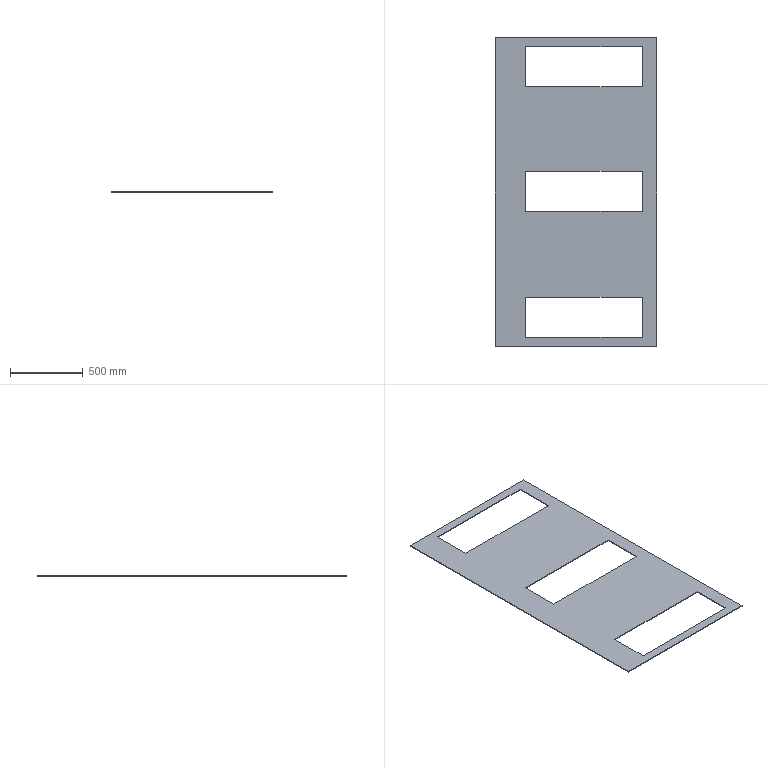Part | SolidWorks | features Extrusion 1 | 1 solid | 18 faces | box 1111 x 2124 x 5 mm | volume 8464783 mm3 | plane 18
STEP:
#1=CARTESIAN_POINT('',(207.052,1206.44,5.));
#2=VERTEX_POINT('',#1);
#3=CARTESIAN_POINT('',(207.052,930.678,5.));
#4=VERTEX_POINT('',#3);
#5=CARTESIAN_POINT('',(207.052,930.678,5.));
#6=DIRECTION('',(0.,-1.,0.));
#7=VECTOR('',#6,1000.);
#8=LINE('',#5,#7);
#9=EDGE_CURVE('',#2,#4,#8,.T.);
#10=ORIENTED_EDGE('',*,*,#9,.F.);
#11=CARTESIAN_POINT('',(1012.074,1206.44,5.));
#12=VERTEX_POINT('',#11);
#13=CARTESIAN_POINT('',(207.052,1206.44,5.));
#14=DIRECTION('',(-1.,0.,0.));
#15=VECTOR('',#14,1000.);
#16=LINE('',#13,#15);
#17=EDGE_CURVE('',#12,#2,#16,.T.);
#18=ORIENTED_EDGE('',*,*,#17,.F.);
#19=CARTESIAN_POINT('',(1012.074,930.678,5.));
#20=VERTEX_POINT('',#19);
#21=CARTESIAN_POINT('',(1012.074,1206.44,5.));
#22=DIRECTION('',(0.,1.,0.));
#23=VECTOR('',#22,1000.);
#24=LINE('',#21,#23);
#25=EDGE_CURVE('',#20,#12,#24,.T.);
#26=ORIENTED_EDGE('',*,*,#25,.F.);
#27=CARTESIAN_POINT('',(1012.074,930.678,5.));
#28=DIRECTION('',(1.,0.,0.));
#29=VECTOR('',#28,1000.);
#30=LINE('',#27,#29);
#31=EDGE_CURVE('',#4,#20,#30,.T.);
#32=ORIENTED_EDGE('',*,*,#31,.F.);
#33=EDGE_LOOP('',(#10,#18,#26,#32));
#34=FACE_BOUND('',#33,.T.);
#35=CARTESIAN_POINT('',(0.,2124.,5.));
#36=VERTEX_POINT('',#35);
#37=CARTESIAN_POINT('',(0.,0.,5.));
#38=VERTEX_POINT('',#37);
#39=CARTESIAN_POINT('',(0.,0.,5.));
#40=DIRECTION('',(0.,-1.,0.));
#41=VECTOR('',#40,1000.);
#42=LINE('',#39,#41);
#43=EDGE_CURVE('',#36,#38,#42,.T.);
#44=ORIENTED_EDGE('',*,*,#43,.T.);
#45=CARTESIAN_POINT('',(1110.612,0.,5.));
#46=VERTEX_POINT('',#45);
#47=CARTESIAN_POINT('',(1110.612,0.,5.));
#48=DIRECTION('',(1.,0.,0.));
#49=VECTOR('',#48,1000.);
#50=LINE('',#47,#49);
#51=EDGE_CURVE('',#38,#46,#50,.T.);
#52=ORIENTED_EDGE('',*,*,#51,.T.);
#53=CARTESIAN_POINT('',(1110.612,2124.,5.));
#54=VERTEX_POINT('',#53);
#55=CARTESIAN_POINT('',(1110.612,2124.,5.));
#56=DIRECTION('',(0.,1.,0.));
#57=VECTOR('',#56,1000.);
#58=LINE('',#55,#57);
#59=EDGE_CURVE('',#46,#54,#58,.T.);
#60=ORIENTED_EDGE('',*,*,#59,.T.);
#61=CARTESIAN_POINT('',(0.,2124.,5.));
#62=DIRECTION('',(-1.,0.,0.));
#63=VECTOR('',#62,1000.);
#64=LINE('',#61,#63);
#65=EDGE_CURVE('',#54,#36,#64,.T.);
#66=ORIENTED_EDGE('',*,*,#65,.T.);
#67=EDGE_LOOP('',(#44,#52,#60,#66));
#68=FACE_OUTER_BOUND('',#67,.T.);
#69=CARTESIAN_POINT('',(207.052,2063.657,5.));
#70=VERTEX_POINT('',#69);
#71=CARTESIAN_POINT('',(207.052,1787.895,5.));
#72=VERTEX_POINT('',#71);
#73=CARTESIAN_POINT('',(207.052,1787.895,5.));
#74=DIRECTION('',(0.,-1.,0.));
#75=VECTOR('',#74,1000.);
#76=LINE('',#73,#75);
#77=EDGE_CURVE('',#70,#72,#76,.T.);
#78=ORIENTED_EDGE('',*,*,#77,.F.);
#79=CARTESIAN_POINT('',(1012.074,2063.657,5.));
#80=VERTEX_POINT('',#79);
#81=CARTESIAN_POINT('',(207.052,2063.657,5.));
#82=DIRECTION('',(-1.,0.,0.));
#83=VECTOR('',#82,1000.);
#84=LINE('',#81,#83);
#85=EDGE_CURVE('',#80,#70,#84,.T.);
#86=ORIENTED_EDGE('',*,*,#85,.F.);
#87=CARTESIAN_POINT('',(1012.074,1787.895,5.));
#88=VERTEX_POINT('',#87);
#89=CARTESIAN_POINT('',(1012.074,2063.657,5.));
#90=DIRECTION('',(0.,1.,0.));
#91=VECTOR('',#90,1000.);
#92=LINE('',#89,#91);
#93=EDGE_CURVE('',#88,#80,#92,.T.);
#94=ORIENTED_EDGE('',*,*,#93,.F.);
#95=CARTESIAN_POINT('',(1012.074,1787.895,5.));
#96=DIRECTION('',(1.,0.,0.));
#97=VECTOR('',#96,1000.);
#98=LINE('',#95,#97);
#99=EDGE_CURVE('',#72,#88,#98,.T.);
#100=ORIENTED_EDGE('',*,*,#99,.F.);
#101=EDGE_LOOP('',(#78,#86,#94,#100));
#102=FACE_BOUND('',#101,.T.);
#103=CARTESIAN_POINT('',(207.052,336.013,5.));
#104=VERTEX_POINT('',#103);
#105=CARTESIAN_POINT('',(207.052,60.251,5.));
#106=VERTEX_POINT('',#105);
#107=CARTESIAN_POINT('',(207.052,60.251,5.));
#108=DIRECTION('',(0.,-1.,0.));
#109=VECTOR('',#108,1000.);
#110=LINE('',#107,#109);
#111=EDGE_CURVE('',#104,#106,#110,.T.);
#112=ORIENTED_EDGE('',*,*,#111,.F.);
#113=CARTESIAN_POINT('',(1012.074,336.013,5.));
#114=VERTEX_POINT('',#113);
#115=CARTESIAN_POINT('',(207.052,336.013,5.));
#116=DIRECTION('',(-1.,0.,0.));
#117=VECTOR('',#116,1000.);
#118=LINE('',#115,#117);
#119=EDGE_CURVE('',#114,#104,#118,.T.);
#120=ORIENTED_EDGE('',*,*,#119,.F.);
#121=CARTESIAN_POINT('',(1012.074,60.251,5.));
#122=VERTEX_POINT('',#121);
#123=CARTESIAN_POINT('',(1012.074,336.013,5.));
#124=DIRECTION('',(0.,1.,0.));
#125=VECTOR('',#124,1000.);
#126=LINE('',#123,#125);
#127=EDGE_CURVE('',#122,#114,#126,.T.);
#128=ORIENTED_EDGE('',*,*,#127,.F.);
#129=CARTESIAN_POINT('',(1012.074,60.251,5.));
#130=DIRECTION('',(1.,0.,0.));
#131=VECTOR('',#130,1000.);
#132=LINE('',#129,#131);
#133=EDGE_CURVE('',#106,#122,#132,.T.);
#134=ORIENTED_EDGE('',*,*,#133,.F.);
#135=EDGE_LOOP('',(#112,#120,#128,#134));
#136=FACE_BOUND('',#135,.T.);
#137=CARTESIAN_POINT('',(0.,0.,5.));
#138=DIRECTION('',(0.,0.,-1.));
#139=DIRECTION('',(-1.,0.,0.));
#140=AXIS2_PLACEMENT_3D('',#137,#138,#139);
#141=PLANE('',#140);
#142=ADVANCED_FACE('',(#34,#68,#102,#136),#141,.F.);
#143=CARTESIAN_POINT('',(0.,2124.,0.));
#144=VERTEX_POINT('',#143);
#145=CARTESIAN_POINT('',(0.,0.,0.));
#146=VERTEX_POINT('',#145);
#147=CARTESIAN_POINT('',(0.,0.,0.));
#148=DIRECTION('',(0.,-1.,0.));
#149=VECTOR('',#148,1000.);
#150=LINE('',#147,#149);
#151=EDGE_CURVE('',#144,#146,#150,.T.);
#152=ORIENTED_EDGE('',*,*,#151,.F.);
#153=CARTESIAN_POINT('',(1110.612,2124.,0.));
#154=VERTEX_POINT('',#153);
#155=CARTESIAN_POINT('',(0.,2124.,0.));
#156=DIRECTION('',(-1.,0.,0.));
#157=VECTOR('',#156,1000.);
#158=LINE('',#155,#157);
#159=EDGE_CURVE('',#154,#144,#158,.T.);
#160=ORIENTED_EDGE('',*,*,#159,.F.);
#161=CARTESIAN_POINT('',(1110.612,0.,0.));
#162=VERTEX_POINT('',#161);
#163=CARTESIAN_POINT('',(1110.612,2124.,0.));
#164=DIRECTION('',(0.,1.,0.));
#165=VECTOR('',#164,1000.);
#166=LINE('',#163,#165);
#167=EDGE_CURVE('',#162,#154,#166,.T.);
#168=ORIENTED_EDGE('',*,*,#167,.F.);
#169=CARTESIAN_POINT('',(1110.612,0.,0.));
#170=DIRECTION('',(1.,0.,0.));
#171=VECTOR('',#170,1000.);
#172=LINE('',#169,#171);
#173=EDGE_CURVE('',#146,#162,#172,.T.);
#174=ORIENTED_EDGE('',*,*,#173,.F.);
#175=EDGE_LOOP('',(#152,#160,#168,#174));
#176=FACE_OUTER_BOUND('',#175,.T.);
#177=CARTESIAN_POINT('',(1012.074,2063.657,0.));
#178=VERTEX_POINT('',#177);
#179=CARTESIAN_POINT('',(207.052,2063.657,0.));
#180=VERTEX_POINT('',#179);
#181=CARTESIAN_POINT('',(207.052,2063.657,0.));
#182=DIRECTION('',(-1.,0.,0.));
#183=VECTOR('',#182,1000.);
#184=LINE('',#181,#183);
#185=EDGE_CURVE('',#178,#180,#184,.T.);
#186=ORIENTED_EDGE('',*,*,#185,.T.);
#187=CARTESIAN_POINT('',(207.052,1787.895,0.));
#188=VERTEX_POINT('',#187);
#189=CARTESIAN_POINT('',(207.052,1787.895,0.));
#190=DIRECTION('',(0.,-1.,0.));
#191=VECTOR('',#190,1000.);
#192=LINE('',#189,#191);
#193=EDGE_CURVE('',#180,#188,#192,.T.);
#194=ORIENTED_EDGE('',*,*,#193,.T.);
#195=CARTESIAN_POINT('',(1012.074,1787.895,0.));
#196=VERTEX_POINT('',#195);
#197=CARTESIAN_POINT('',(1012.074,1787.895,0.));
#198=DIRECTION('',(1.,0.,0.));
#199=VECTOR('',#198,1000.);
#200=LINE('',#197,#199);
#201=EDGE_CURVE('',#188,#196,#200,.T.);
#202=ORIENTED_EDGE('',*,*,#201,.T.);
#203=CARTESIAN_POINT('',(1012.074,2063.657,0.));
#204=DIRECTION('',(0.,1.,0.));
#205=VECTOR('',#204,1000.);
#206=LINE('',#203,#205);
#207=EDGE_CURVE('',#196,#178,#206,.T.);
#208=ORIENTED_EDGE('',*,*,#207,.T.);
#209=EDGE_LOOP('',(#186,#194,#202,#208));
#210=FACE_BOUND('',#209,.T.);
#211=CARTESIAN_POINT('',(1012.074,1206.44,0.));
#212=VERTEX_POINT('',#211);
#213=CARTESIAN_POINT('',(207.052,1206.44,0.));
#214=VERTEX_POINT('',#213);
#215=CARTESIAN_POINT('',(207.052,1206.44,0.));
#216=DIRECTION('',(-1.,0.,0.));
#217=VECTOR('',#216,1000.);
#218=LINE('',#215,#217);
#219=EDGE_CURVE('',#212,#214,#218,.T.);
#220=ORIENTED_EDGE('',*,*,#219,.T.);
#221=CARTESIAN_POINT('',(207.052,930.678,0.));
#222=VERTEX_POINT('',#221);
#223=CARTESIAN_POINT('',(207.052,930.678,0.));
#224=DIRECTION('',(0.,-1.,0.));
#225=VECTOR('',#224,1000.);
#226=LINE('',#223,#225);
#227=EDGE_CURVE('',#214,#222,#226,.T.);
#228=ORIENTED_EDGE('',*,*,#227,.T.);
#229=CARTESIAN_POINT('',(1012.074,930.678,0.));
#230=VERTEX_POINT('',#229);
#231=CARTESIAN_POINT('',(1012.074,930.678,0.));
#232=DIRECTION('',(1.,0.,0.));
#233=VECTOR('',#232,1000.);
#234=LINE('',#231,#233);
#235=EDGE_CURVE('',#222,#230,#234,.T.);
#236=ORIENTED_EDGE('',*,*,#235,.T.);
#237=CARTESIAN_POINT('',(1012.074,1206.44,0.));
#238=DIRECTION('',(0.,1.,0.));
#239=VECTOR('',#238,1000.);
#240=LINE('',#237,#239);
#241=EDGE_CURVE('',#230,#212,#240,.T.);
#242=ORIENTED_EDGE('',*,*,#241,.T.);
#243=EDGE_LOOP('',(#220,#228,#236,#242));
#244=FACE_BOUND('',#243,.T.);
#245=CARTESIAN_POINT('',(1012.074,336.013,0.));
#246=VERTEX_POINT('',#245);
#247=CARTESIAN_POINT('',(207.052,336.013,0.));
#248=VERTEX_POINT('',#247);
#249=CARTESIAN_POINT('',(207.052,336.013,0.));
#250=DIRECTION('',(-1.,0.,0.));
#251=VECTOR('',#250,1000.);
#252=LINE('',#249,#251);
#253=EDGE_CURVE('',#246,#248,#252,.T.);
#254=ORIENTED_EDGE('',*,*,#253,.T.);
#255=CARTESIAN_POINT('',(207.052,60.251,0.));
#256=VERTEX_POINT('',#255);
#257=CARTESIAN_POINT('',(207.052,60.251,0.));
#258=DIRECTION('',(0.,-1.,0.));
#259=VECTOR('',#258,1000.);
#260=LINE('',#257,#259);
#261=EDGE_CURVE('',#248,#256,#260,.T.);
#262=ORIENTED_EDGE('',*,*,#261,.T.);
#263=CARTESIAN_POINT('',(1012.074,60.251,0.));
#264=VERTEX_POINT('',#263);
#265=CARTESIAN_POINT('',(1012.074,60.251,0.));
#266=DIRECTION('',(1.,0.,0.));
#267=VECTOR('',#266,1000.);
#268=LINE('',#265,#267);
#269=EDGE_CURVE('',#256,#264,#268,.T.);
#270=ORIENTED_EDGE('',*,*,#269,.T.);
#271=CARTESIAN_POINT('',(1012.074,336.013,0.));
#272=DIRECTION('',(0.,1.,0.));
#273=VECTOR('',#272,1000.);
#274=LINE('',#271,#273);
#275=EDGE_CURVE('',#264,#246,#274,.T.);
#276=ORIENTED_EDGE('',*,*,#275,.T.);
#277=EDGE_LOOP('',(#254,#262,#270,#276));
#278=FACE_BOUND('',#277,.T.);
#279=CARTESIAN_POINT('',(0.,0.,0.));
#280=DIRECTION('',(0.,0.,-1.));
#281=DIRECTION('',(-1.,0.,0.));
#282=AXIS2_PLACEMENT_3D('',#279,#280,#281);
#283=PLANE('',#282);
#284=ADVANCED_FACE('',(#176,#210,#244,#278),#283,.T.);
#285=ORIENTED_EDGE('',*,*,#151,.T.);
#286=CARTESIAN_POINT('',(0.,0.,5.));
#287=DIRECTION('',(0.,0.,-1.));
#288=VECTOR('',#287,1000.);
#289=LINE('',#286,#288);
#290=EDGE_CURVE('',#38,#146,#289,.T.);
#291=ORIENTED_EDGE('',*,*,#290,.F.);
#292=ORIENTED_EDGE('',*,*,#43,.F.);
#293=CARTESIAN_POINT('',(0.,2124.,5.));
#294=DIRECTION('',(0.,0.,-1.));
#295=VECTOR('',#294,1000.);
#296=LINE('',#293,#295);
#297=EDGE_CURVE('',#36,#144,#296,.T.);
#298=ORIENTED_EDGE('',*,*,#297,.T.);
#299=EDGE_LOOP('',(#285,#291,#292,#298));
#300=FACE_OUTER_BOUND('',#299,.T.);
#301=CARTESIAN_POINT('',(0.,0.,5.));
#302=DIRECTION('',(1.,0.,0.));
#303=DIRECTION('',(0.,0.,-1.));
#304=AXIS2_PLACEMENT_3D('',#301,#302,#303);
#305=PLANE('',#304);
#306=ADVANCED_FACE('',(#300),#305,.F.);
#307=ORIENTED_EDGE('',*,*,#173,.T.);
#308=CARTESIAN_POINT('',(1110.612,0.,5.));
#309=DIRECTION('',(0.,0.,-1.));
#310=VECTOR('',#309,1000.);
#311=LINE('',#308,#310);
#312=EDGE_CURVE('',#46,#162,#311,.T.);
#313=ORIENTED_EDGE('',*,*,#312,.F.);
#314=ORIENTED_EDGE('',*,*,#51,.F.);
#315=ORIENTED_EDGE('',*,*,#290,.T.);
#316=EDGE_LOOP('',(#307,#313,#314,#315));
#317=FACE_OUTER_BOUND('',#316,.T.);
#318=CARTESIAN_POINT('',(1110.612,0.,5.));
#319=DIRECTION('',(0.,1.,0.));
#320=DIRECTION('',(0.,0.,1.));
#321=AXIS2_PLACEMENT_3D('',#318,#319,#320);
#322=PLANE('',#321);
#323=ADVANCED_FACE('',(#317),#322,.F.);
#324=ORIENTED_EDGE('',*,*,#167,.T.);
#325=CARTESIAN_POINT('',(1110.612,2124.,5.));
#326=DIRECTION('',(0.,0.,-1.));
#327=VECTOR('',#326,1000.);
#328=LINE('',#325,#327);
#329=EDGE_CURVE('',#54,#154,#328,.T.);
#330=ORIENTED_EDGE('',*,*,#329,.F.);
#331=ORIENTED_EDGE('',*,*,#59,.F.);
#332=ORIENTED_EDGE('',*,*,#312,.T.);
#333=EDGE_LOOP('',(#324,#330,#331,#332));
#334=FACE_OUTER_BOUND('',#333,.T.);
#335=CARTESIAN_POINT('',(1110.612,2124.,5.));
#336=DIRECTION('',(-1.,0.,0.));
#337=DIRECTION('',(0.,0.,1.));
#338=AXIS2_PLACEMENT_3D('',#335,#336,#337);
#339=PLANE('',#338);
#340=ADVANCED_FACE('',(#334),#339,.F.);
#341=ORIENTED_EDGE('',*,*,#159,.T.);
#342=ORIENTED_EDGE('',*,*,#297,.F.);
#343=ORIENTED_EDGE('',*,*,#65,.F.);
#344=ORIENTED_EDGE('',*,*,#329,.T.);
#345=EDGE_LOOP('',(#341,#342,#343,#344));
#346=FACE_OUTER_BOUND('',#345,.T.);
#347=CARTESIAN_POINT('',(0.,2124.,5.));
#348=DIRECTION('',(0.,-1.,0.));
#349=DIRECTION('',(0.,0.,-1.));
#350=AXIS2_PLACEMENT_3D('',#347,#348,#349);
#351=PLANE('',#350);
#352=ADVANCED_FACE('',(#346),#351,.F.);
#353=ORIENTED_EDGE('',*,*,#193,.F.);
#354=CARTESIAN_POINT('',(207.052,2063.657,5.));
#355=DIRECTION('',(0.,0.,-1.));
#356=VECTOR('',#355,1000.);
#357=LINE('',#354,#356);
#358=EDGE_CURVE('',#70,#180,#357,.T.);
#359=ORIENTED_EDGE('',*,*,#358,.F.);
#360=ORIENTED_EDGE('',*,*,#77,.T.);
#361=CARTESIAN_POINT('',(207.052,1787.895,5.));
#362=DIRECTION('',(0.,0.,-1.));
#363=VECTOR('',#362,1000.);
#364=LINE('',#361,#363);
#365=EDGE_CURVE('',#72,#188,#364,.T.);
#366=ORIENTED_EDGE('',*,*,#365,.T.);
#367=EDGE_LOOP('',(#353,#359,#360,#366));
#368=FACE_OUTER_BOUND('',#367,.T.);
#369=CARTESIAN_POINT('',(207.052,1787.895,5.));
#370=DIRECTION('',(1.,0.,0.));
#371=DIRECTION('',(0.,0.,-1.));
#372=AXIS2_PLACEMENT_3D('',#369,#370,#371);
#373=PLANE('',#372);
#374=ADVANCED_FACE('',(#368),#373,.T.);
#375=ORIENTED_EDGE('',*,*,#201,.F.);
#376=ORIENTED_EDGE('',*,*,#365,.F.);
#377=ORIENTED_EDGE('',*,*,#99,.T.);
#378=CARTESIAN_POINT('',(1012.074,1787.895,5.));
#379=DIRECTION('',(0.,0.,-1.));
#380=VECTOR('',#379,1000.);
#381=LINE('',#378,#380);
#382=EDGE_CURVE('',#88,#196,#381,.T.);
#383=ORIENTED_EDGE('',*,*,#382,.T.);
#384=EDGE_LOOP('',(#375,#376,#377,#383));
#385=FACE_OUTER_BOUND('',#384,.T.);
#386=CARTESIAN_POINT('',(1012.074,1787.895,5.));
#387=DIRECTION('',(0.,1.,0.));
#388=DIRECTION('',(0.,0.,1.));
#389=AXIS2_PLACEMENT_3D('',#386,#387,#388);
#390=PLANE('',#389);
#391=ADVANCED_FACE('',(#385),#390,.T.);
#392=ORIENTED_EDGE('',*,*,#207,.F.);
#393=ORIENTED_EDGE('',*,*,#382,.F.);
#394=ORIENTED_EDGE('',*,*,#93,.T.);
#395=CARTESIAN_POINT('',(1012.074,2063.657,5.));
#396=DIRECTION('',(0.,0.,-1.));
#397=VECTOR('',#396,1000.);
#398=LINE('',#395,#397);
#399=EDGE_CURVE('',#80,#178,#398,.T.);
#400=ORIENTED_EDGE('',*,*,#399,.T.);
#401=EDGE_LOOP('',(#392,#393,#394,#400));
#402=FACE_OUTER_BOUND('',#401,.T.);
#403=CARTESIAN_POINT('',(1012.074,2063.657,5.));
#404=DIRECTION('',(-1.,0.,0.));
#405=DIRECTION('',(0.,0.,1.));
#406=AXIS2_PLACEMENT_3D('',#403,#404,#405);
#407=PLANE('',#406);
#408=ADVANCED_FACE('',(#402),#407,.T.);
#409=ORIENTED_EDGE('',*,*,#185,.F.);
#410=ORIENTED_EDGE('',*,*,#399,.F.);
#411=ORIENTED_EDGE('',*,*,#85,.T.);
#412=ORIENTED_EDGE('',*,*,#358,.T.);
#413=EDGE_LOOP('',(#409,#410,#411,#412));
#414=FACE_OUTER_BOUND('',#413,.T.);
#415=CARTESIAN_POINT('',(207.052,2063.657,5.));
#416=DIRECTION('',(0.,-1.,0.));
#417=DIRECTION('',(0.,0.,-1.));
#418=AXIS2_PLACEMENT_3D('',#415,#416,#417);
#419=PLANE('',#418);
#420=ADVANCED_FACE('',(#414),#419,.T.);
#421=ORIENTED_EDGE('',*,*,#227,.F.);
#422=CARTESIAN_POINT('',(207.052,1206.44,5.));
#423=DIRECTION('',(0.,0.,-1.));
#424=VECTOR('',#423,1000.);
#425=LINE('',#422,#424);
#426=EDGE_CURVE('',#2,#214,#425,.T.);
#427=ORIENTED_EDGE('',*,*,#426,.F.);
#428=ORIENTED_EDGE('',*,*,#9,.T.);
#429=CARTESIAN_POINT('',(207.052,930.678,5.));
#430=DIRECTION('',(0.,0.,-1.));
#431=VECTOR('',#430,1000.);
#432=LINE('',#429,#431);
#433=EDGE_CURVE('',#4,#222,#432,.T.);
#434=ORIENTED_EDGE('',*,*,#433,.T.);
#435=EDGE_LOOP('',(#421,#427,#428,#434));
#436=FACE_OUTER_BOUND('',#435,.T.);
#437=CARTESIAN_POINT('',(207.052,930.678,5.));
#438=DIRECTION('',(1.,0.,0.));
#439=DIRECTION('',(0.,0.,-1.));
#440=AXIS2_PLACEMENT_3D('',#437,#438,#439);
#441=PLANE('',#440);
#442=ADVANCED_FACE('',(#436),#441,.T.);
#443=ORIENTED_EDGE('',*,*,#235,.F.);
#444=ORIENTED_EDGE('',*,*,#433,.F.);
#445=ORIENTED_EDGE('',*,*,#31,.T.);
#446=CARTESIAN_POINT('',(1012.074,930.678,5.));
#447=DIRECTION('',(0.,0.,-1.));
#448=VECTOR('',#447,1000.);
#449=LINE('',#446,#448);
#450=EDGE_CURVE('',#20,#230,#449,.T.);
#451=ORIENTED_EDGE('',*,*,#450,.T.);
#452=EDGE_LOOP('',(#443,#444,#445,#451));
#453=FACE_OUTER_BOUND('',#452,.T.);
#454=CARTESIAN_POINT('',(1012.074,930.678,5.));
#455=DIRECTION('',(0.,1.,0.));
#456=DIRECTION('',(0.,0.,1.));
#457=AXIS2_PLACEMENT_3D('',#454,#455,#456);
#458=PLANE('',#457);
#459=ADVANCED_FACE('',(#453),#458,.T.);
#460=ORIENTED_EDGE('',*,*,#241,.F.);
#461=ORIENTED_EDGE('',*,*,#450,.F.);
#462=ORIENTED_EDGE('',*,*,#25,.T.);
#463=CARTESIAN_POINT('',(1012.074,1206.44,5.));
#464=DIRECTION('',(0.,0.,-1.));
#465=VECTOR('',#464,1000.);
#466=LINE('',#463,#465);
#467=EDGE_CURVE('',#12,#212,#466,.T.);
#468=ORIENTED_EDGE('',*,*,#467,.T.);
#469=EDGE_LOOP('',(#460,#461,#462,#468));
#470=FACE_OUTER_BOUND('',#469,.T.);
#471=CARTESIAN_POINT('',(1012.074,1206.44,5.));
#472=DIRECTION('',(-1.,0.,0.));
#473=DIRECTION('',(0.,0.,1.));
#474=AXIS2_PLACEMENT_3D('',#471,#472,#473);
#475=PLANE('',#474);
#476=ADVANCED_FACE('',(#470),#475,.T.);
#477=ORIENTED_EDGE('',*,*,#219,.F.);
#478=ORIENTED_EDGE('',*,*,#467,.F.);
#479=ORIENTED_EDGE('',*,*,#17,.T.);
#480=ORIENTED_EDGE('',*,*,#426,.T.);
#481=EDGE_LOOP('',(#477,#478,#479,#480));
#482=FACE_OUTER_BOUND('',#481,.T.);
#483=CARTESIAN_POINT('',(207.052,1206.44,5.));
#484=DIRECTION('',(0.,-1.,0.));
#485=DIRECTION('',(0.,0.,-1.));
#486=AXIS2_PLACEMENT_3D('',#483,#484,#485);
#487=PLANE('',#486);
#488=ADVANCED_FACE('',(#482),#487,.T.);
#489=ORIENTED_EDGE('',*,*,#261,.F.);
#490=CARTESIAN_POINT('',(207.052,336.013,5.));
#491=DIRECTION('',(0.,0.,-1.));
#492=VECTOR('',#491,1000.);
#493=LINE('',#490,#492);
#494=EDGE_CURVE('',#104,#248,#493,.T.);
#495=ORIENTED_EDGE('',*,*,#494,.F.);
#496=ORIENTED_EDGE('',*,*,#111,.T.);
#497=CARTESIAN_POINT('',(207.052,60.251,5.));
#498=DIRECTION('',(0.,0.,-1.));
#499=VECTOR('',#498,1000.);
#500=LINE('',#497,#499);
#501=EDGE_CURVE('',#106,#256,#500,.T.);
#502=ORIENTED_EDGE('',*,*,#501,.T.);
#503=EDGE_LOOP('',(#489,#495,#496,#502));
#504=FACE_OUTER_BOUND('',#503,.T.);
#505=CARTESIAN_POINT('',(207.052,60.251,5.));
#506=DIRECTION('',(1.,0.,0.));
#507=DIRECTION('',(0.,0.,-1.));
#508=AXIS2_PLACEMENT_3D('',#505,#506,#507);
#509=PLANE('',#508);
#510=ADVANCED_FACE('',(#504),#509,.T.);
#511=ORIENTED_EDGE('',*,*,#269,.F.);
#512=ORIENTED_EDGE('',*,*,#501,.F.);
#513=ORIENTED_EDGE('',*,*,#133,.T.);
#514=CARTESIAN_POINT('',(1012.074,60.251,5.));
#515=DIRECTION('',(0.,0.,-1.));
#516=VECTOR('',#515,1000.);
#517=LINE('',#514,#516);
#518=EDGE_CURVE('',#122,#264,#517,.T.);
#519=ORIENTED_EDGE('',*,*,#518,.T.);
#520=EDGE_LOOP('',(#511,#512,#513,#519));
#521=FACE_OUTER_BOUND('',#520,.T.);
#522=CARTESIAN_POINT('',(1012.074,60.251,5.));
#523=DIRECTION('',(0.,1.,0.));
#524=DIRECTION('',(0.,0.,1.));
#525=AXIS2_PLACEMENT_3D('',#522,#523,#524);
#526=PLANE('',#525);
#527=ADVANCED_FACE('',(#521),#526,.T.);
#528=ORIENTED_EDGE('',*,*,#275,.F.);
#529=ORIENTED_EDGE('',*,*,#518,.F.);
#530=ORIENTED_EDGE('',*,*,#127,.T.);
#531=CARTESIAN_POINT('',(1012.074,336.013,5.));
#532=DIRECTION('',(0.,0.,-1.));
#533=VECTOR('',#532,1000.);
#534=LINE('',#531,#533);
#535=EDGE_CURVE('',#114,#246,#534,.T.);
#536=ORIENTED_EDGE('',*,*,#535,.T.);
#537=EDGE_LOOP('',(#528,#529,#530,#536));
#538=FACE_OUTER_BOUND('',#537,.T.);
#539=CARTESIAN_POINT('',(1012.074,336.013,5.));
#540=DIRECTION('',(-1.,0.,0.));
#541=DIRECTION('',(0.,0.,1.));
#542=AXIS2_PLACEMENT_3D('',#539,#540,#541);
#543=PLANE('',#542);
#544=ADVANCED_FACE('',(#538),#543,.T.);
#545=ORIENTED_EDGE('',*,*,#253,.F.);
#546=ORIENTED_EDGE('',*,*,#535,.F.);
#547=ORIENTED_EDGE('',*,*,#119,.T.);
#548=ORIENTED_EDGE('',*,*,#494,.T.);
#549=EDGE_LOOP('',(#545,#546,#547,#548));
#550=FACE_OUTER_BOUND('',#549,.T.);
#551=CARTESIAN_POINT('',(207.052,336.013,5.));
#552=DIRECTION('',(0.,-1.,0.));
#553=DIRECTION('',(0.,0.,-1.));
#554=AXIS2_PLACEMENT_3D('',#551,#552,#553);
#555=PLANE('',#554);
#556=ADVANCED_FACE('',(#550),#555,.T.);
#557=CLOSED_SHELL('',(#142,#284,#306,#323,#340,#352,#374,#391,#408,#420,#442,#459,#476,#488,#510,#527,#544,#556));
#558=MANIFOLD_SOLID_BREP('',#557);
#559=CARTESIAN_POINT('',(0.,0.,0.));
#560=DIRECTION('',(0.,0.,1.));
#561=DIRECTION('',(1.,0.,0.));
#562=AXIS2_PLACEMENT_3D('',#559,#560,#561);
#563=(LENGTH_UNIT()NAMED_UNIT(*)SI_UNIT(.MILLI.,.METRE.));
#564=UNCERTAINTY_MEASURE_WITH_UNIT(LENGTH_MEASURE(0.00001),#563,'','');
#565=(NAMED_UNIT(*)PLANE_ANGLE_UNIT()SI_UNIT($,.RADIAN.));
#566=(NAMED_UNIT(*)SI_UNIT($,.STERADIAN.)SOLID_ANGLE_UNIT());
#567=(GEOMETRIC_REPRESENTATION_CONTEXT(3)GLOBAL_UNCERTAINTY_ASSIGNED_CONTEXT((#564))GLOBAL_UNIT_ASSIGNED_CONTEXT((#563,#565,#566))REPRESENTATION_CONTEXT('',''));
#568=ADVANCED_BREP_SHAPE_REPRESENTATION('',(#558,#562),#567);